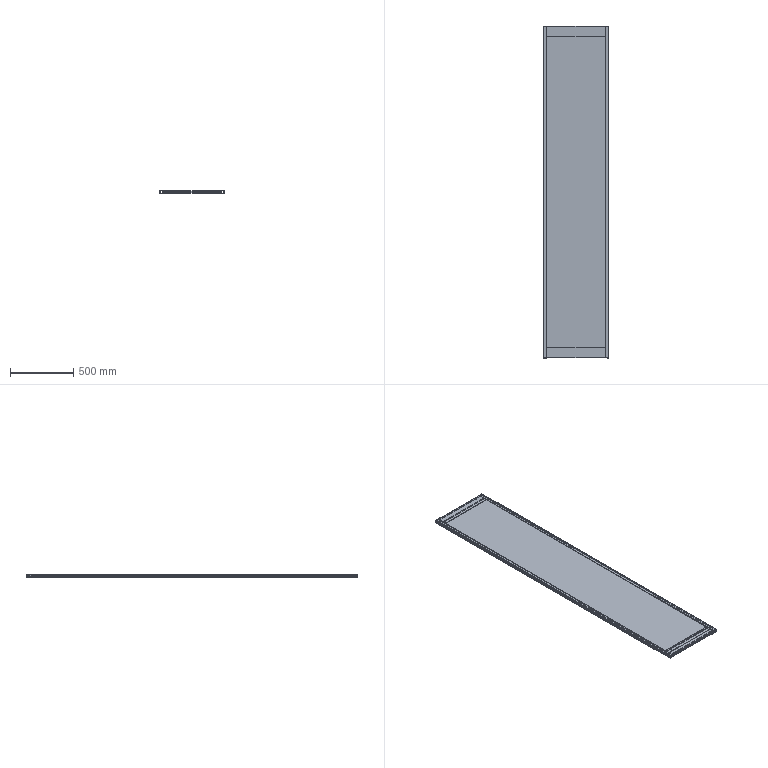Part | 5 solids | 365 faces | box 520 x 2616 x 20.2 mm | volume 13387124 mm3 | cylinder 191 | plane 174 | commonest cylinder face diameters 0.6 x48 13 x48 0.4 x34 1 x21 9 x16 7.2 x12